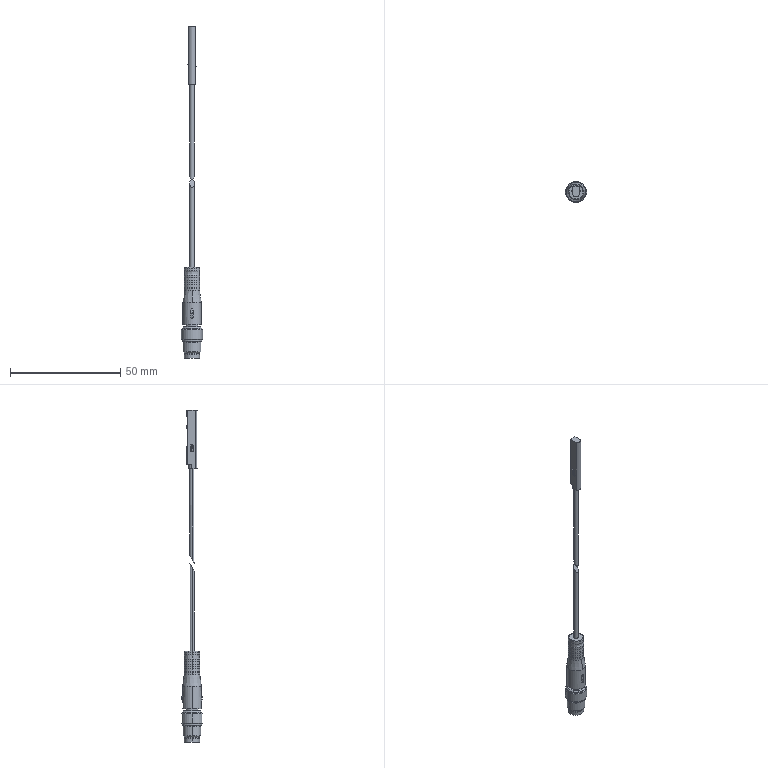Part | SolidWorks | features Attribute 301, BaseBody 5, ICE 1 | 2 solids | 175 faces | box 9.6 x 9.6 x 150.7 mm | volume 2540 mm3 | plane 80 | cylinder 59 | cone 20 | spline 16 | commonest cylinder face diameters 7 x10 1 x6 0.6 x4 2.15 x4 9 x4 2.9 x3